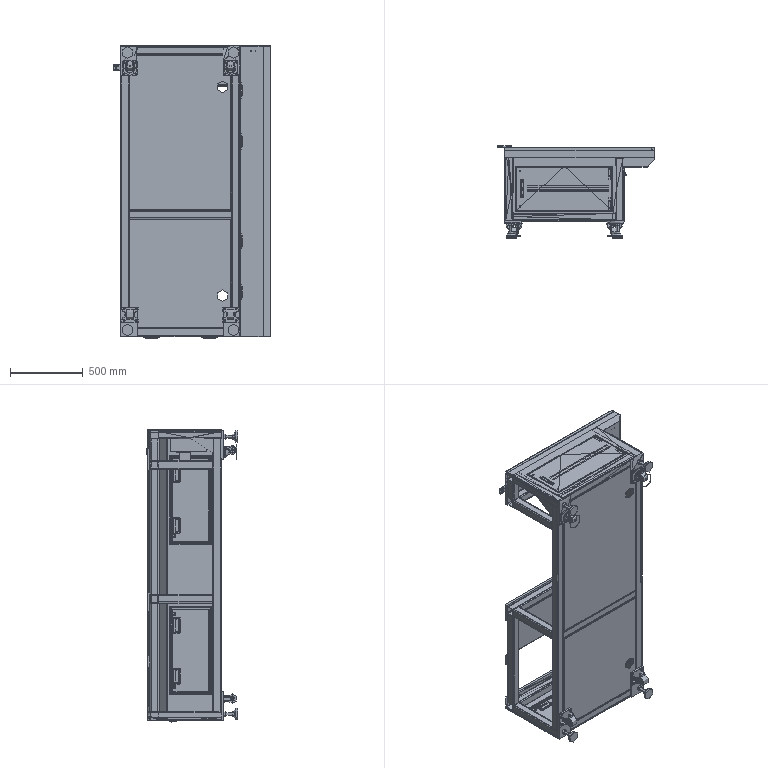Part | NX | features BREP 54 | 74 solids | 3992 faces | volume 10874945838594615770571199719241102023102021036638033925255301972891974279390855974746685811784851390464 mm3 | plane 1861 | cylinder 1506 | cone 247 | torus 222 | spline 156 | commonest cylinder face diameters 4 x160 8 x144 7 x143 10 x104 6 x94 16 x93